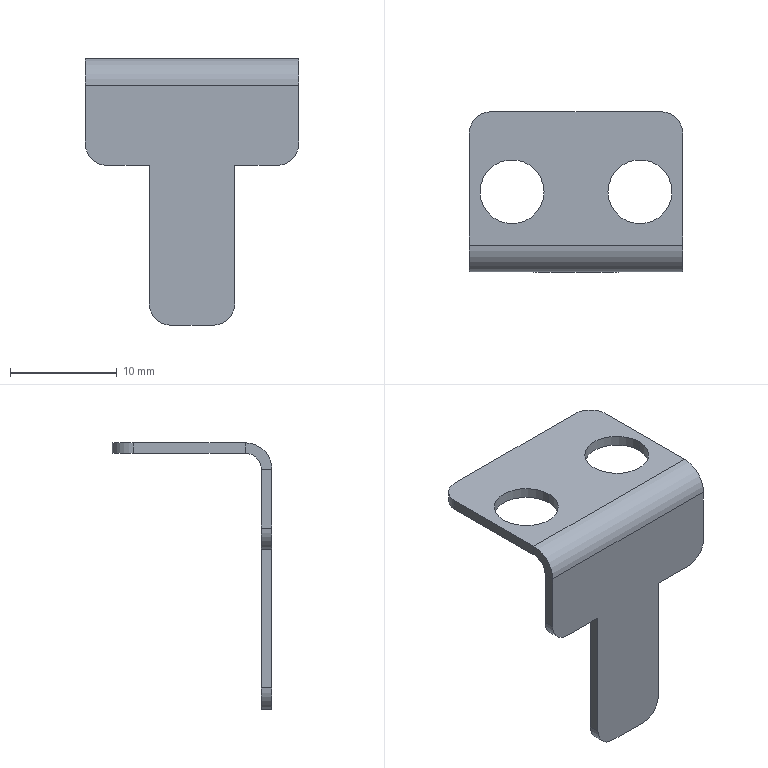Part | STEP file | PN_0018 Sensor DOG_Default | 1 solid | 28 faces | box 20 x 15 x 25 mm | volume 521.133 mm3 | plane 16 | cylinder 12 | commonest cylinder face diameters 4 x6 6 x4 3 x1 5 x1